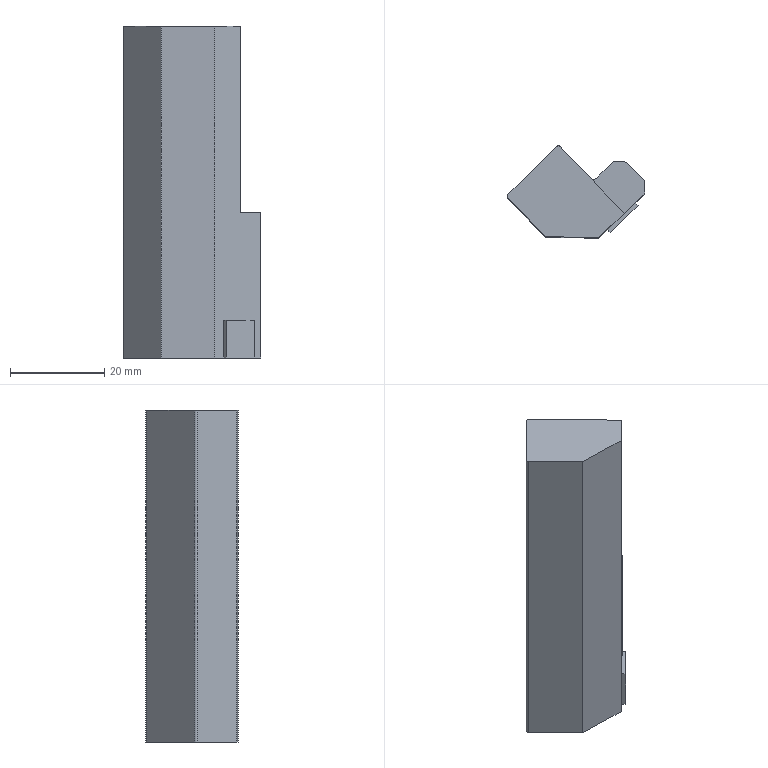Part | STEP file | gslz 2016.10.28-13_id1662_x_t | 1 solid | 19 faces | box 29.227 x 19.541 x 70.5 mm | volume 21986 mm3 | plane 16 | cylinder 3 | commonest cylinder face diameters 1 x2 2 x1
STEP:
#1=CARTESIAN_POINT('',(0.,0.,0.));
#2=DIRECTION('',(0.,0.,1.));
#3=DIRECTION('',(1.,0.,0.));
#4=AXIS2_PLACEMENT_3D('',#1,#2,#3);
#5=CARTESIAN_POINT('',(612.182,-228.399,-23.5));
#6=VERTEX_POINT('',#5);
#7=CARTESIAN_POINT('',(604.209,-220.085,-23.5));
#8=VERTEX_POINT('',#7);
#9=CARTESIAN_POINT('',(645.405,-263.044,-23.5));
#10=DIRECTION('',(-0.6921,0.7218,0.));
#11=VECTOR('',#10,1.);
#12=LINE('',#9,#11);
#13=CARTESIAN_POINT('',(-997.948,1450.63,-27.));
#14=DIRECTION('',(0.7218,0.6921,0.));
#15=DIRECTION('',(-0.6921,0.7218,0.));
#16=AXIS2_PLACEMENT_3D('',#13,#14,#15);
#17=PLANE('',#16);
#18=CARTESIAN_POINT('',(-2374.297,3.5));
#19=DIRECTION('',(1.,0.));
#20=VECTOR('',#19,1.);
#21=LINE('',#18,#20);
#22=(GEOMETRIC_REPRESENTATION_CONTEXT(2)PARAMETRIC_REPRESENTATION_CONTEXT()REPRESENTATION_CONTEXT('',''));
#23=DEFINITIONAL_REPRESENTATION('',(#21),#22);
#24=PCURVE('',#17,#23);
#25=CARTESIAN_POINT('',(467.733,-433.425,-23.5));
#26=DIRECTION('',(0.,0.,1.));
#27=DIRECTION('',(1.,0.,0.));
#28=AXIS2_PLACEMENT_3D('',#25,#26,#27);
#29=PLANE('',#28);
#30=CARTESIAN_POINT('',(177.672,170.382));
#31=DIRECTION('',(-0.6921,0.7218));
#32=VECTOR('',#31,1.);
#33=LINE('',#30,#32);
#34=(GEOMETRIC_REPRESENTATION_CONTEXT(2)PARAMETRIC_REPRESENTATION_CONTEXT()REPRESENTATION_CONTEXT('',''));
#35=DEFINITIONAL_REPRESENTATION('',(#33),#34);
#36=PCURVE('',#29,#35);
#37=SURFACE_CURVE('',#12,(#24,#36),.PCURVE_S1.);
#38=EDGE_CURVE('',#6,#8,#37,.T.);
#39=ORIENTED_EDGE('',*,*,#38,.T.);
#40=CARTESIAN_POINT('',(604.209,-220.085,-94.));
#41=VERTEX_POINT('',#40);
#42=CARTESIAN_POINT('',(604.209,-220.085,-94.));
#43=DIRECTION('',(0.,0.,-1.));
#44=VECTOR('',#43,1.);
#45=LINE('',#42,#44);
#46=CARTESIAN_POINT('',(-2314.777,-67.));
#47=DIRECTION('',(0.,-1.));
#48=VECTOR('',#47,1.);
#49=LINE('',#46,#48);
#50=(GEOMETRIC_REPRESENTATION_CONTEXT(2)PARAMETRIC_REPRESENTATION_CONTEXT()REPRESENTATION_CONTEXT('',''));
#51=DEFINITIONAL_REPRESENTATION('',(#49),#50);
#52=PCURVE('',#17,#51);
#53=CARTESIAN_POINT('',(604.57,-219.739,-116.74));
#54=DIRECTION('',(0.,0.,-1.));
#55=DIRECTION('',(-1.,0.,0.));
#56=AXIS2_PLACEMENT_3D('',#53,#54,#55);
#57=CYLINDRICAL_SURFACE('',#56,0.5);
#58=CARTESIAN_POINT('',(-0.7645,-22.74));
#59=DIRECTION('',(0.,1.));
#60=VECTOR('',#59,1.);
#61=LINE('',#58,#60);
#62=(GEOMETRIC_REPRESENTATION_CONTEXT(2)PARAMETRIC_REPRESENTATION_CONTEXT()REPRESENTATION_CONTEXT('',''));
#63=DEFINITIONAL_REPRESENTATION('',(#61),#62);
#64=PCURVE('',#57,#63);
#65=SURFACE_CURVE('',#45,(#52,#64),.PCURVE_S1.);
#66=EDGE_CURVE('',#8,#41,#65,.T.);
#67=ORIENTED_EDGE('',*,*,#66,.T.);
#68=CARTESIAN_POINT('',(612.182,-228.399,-94.));
#69=VERTEX_POINT('',#68);
#70=CARTESIAN_POINT('',(26.482,382.364,-94.));
#71=DIRECTION('',(-0.6921,0.7218,0.));
#72=VECTOR('',#71,1.);
#73=LINE('',#70,#72);
#74=CARTESIAN_POINT('',(-1480.084,-67.));
#75=DIRECTION('',(1.,0.));
#76=VECTOR('',#75,1.);
#77=LINE('',#74,#76);
#78=(GEOMETRIC_REPRESENTATION_CONTEXT(2)PARAMETRIC_REPRESENTATION_CONTEXT()REPRESENTATION_CONTEXT('',''));
#79=DEFINITIONAL_REPRESENTATION('',(#77),#78);
#80=PCURVE('',#17,#79);
#81=CARTESIAN_POINT('',(-151.191,211.982,-94.));
#82=DIRECTION('',(0.,0.,1.));
#83=DIRECTION('',(1.,0.,0.));
#84=AXIS2_PLACEMENT_3D('',#81,#82,#83);
#85=PLANE('',#84);
#86=CARTESIAN_POINT('',(177.672,170.382));
#87=DIRECTION('',(-0.6921,0.7218));
#88=VECTOR('',#87,1.);
#89=LINE('',#86,#88);
#90=(GEOMETRIC_REPRESENTATION_CONTEXT(2)PARAMETRIC_REPRESENTATION_CONTEXT()REPRESENTATION_CONTEXT('',''));
#91=DEFINITIONAL_REPRESENTATION('',(#89),#90);
#92=PCURVE('',#85,#91);
#93=SURFACE_CURVE('',#73,(#80,#92),.PCURVE_S1.);
#94=EDGE_CURVE('',#69,#41,#93,.T.);
#95=ORIENTED_EDGE('',*,*,#94,.F.);
#96=CARTESIAN_POINT('',(612.182,-228.399,-23.5));
#97=DIRECTION('',(0.,0.,1.));
#98=VECTOR('',#97,1.);
#99=LINE('',#96,#98);
#100=CARTESIAN_POINT('',(-2326.297,3.5));
#101=DIRECTION('',(0.,1.));
#102=VECTOR('',#101,1.);
#103=LINE('',#100,#102);
#104=(GEOMETRIC_REPRESENTATION_CONTEXT(2)PARAMETRIC_REPRESENTATION_CONTEXT()REPRESENTATION_CONTEXT('',''));
#105=DEFINITIONAL_REPRESENTATION('',(#103),#104);
#106=PCURVE('',#17,#105);
#107=CARTESIAN_POINT('',(612.182,-228.399,-27.));
#108=DIRECTION('',(-0.02094,-0.9998,0.));
#109=DIRECTION('',(0.,0.,-1.));
#110=AXIS2_PLACEMENT_3D('',#107,#108,#109);
#111=PLANE('',#110);
#112=CARTESIAN_POINT('',(-3.5,0.));
#113=DIRECTION('',(-1.,0.));
#114=VECTOR('',#113,1.);
#115=LINE('',#112,#114);
#116=(GEOMETRIC_REPRESENTATION_CONTEXT(2)PARAMETRIC_REPRESENTATION_CONTEXT()REPRESENTATION_CONTEXT('',''));
#117=DEFINITIONAL_REPRESENTATION('',(#115),#116);
#118=PCURVE('',#111,#117);
#119=SURFACE_CURVE('',#99,(#106,#118),.PCURVE_S1.);
#120=EDGE_CURVE('',#69,#6,#119,.T.);
#121=ORIENTED_EDGE('',*,*,#120,.T.);
#122=EDGE_LOOP('',(#39,#67,#95,#121));
#123=FACE_BOUND('',#122,.T.);
#124=ADVANCED_FACE('',(#123),#17,.F.);
#125=CARTESIAN_POINT('',(604.22,-219.381,-94.));
#126=VERTEX_POINT('',#125);
#127=CARTESIAN_POINT('',(604.57,-219.739,-94.));
#128=DIRECTION('',(0.,0.,-1.));
#129=DIRECTION('',(1.,0.,0.));
#130=AXIS2_PLACEMENT_3D('',#127,#128,#129);
#131=CIRCLE('',#130,0.5);
#132=CARTESIAN_POINT('',(-3.142,-22.74));
#133=DIRECTION('',(1.,0.));
#134=VECTOR('',#133,1.);
#135=LINE('',#132,#134);
#136=(GEOMETRIC_REPRESENTATION_CONTEXT(2)PARAMETRIC_REPRESENTATION_CONTEXT()REPRESENTATION_CONTEXT('',''));
#137=DEFINITIONAL_REPRESENTATION('',(#135),#136);
#138=PCURVE('',#57,#137);
#139=CARTESIAN_POINT('',(756.261,-431.721));
#140=CARTESIAN_POINT('',(756.261,-432.587));
#141=CARTESIAN_POINT('',(755.511,-432.154));
#142=CARTESIAN_POINT('',(754.761,-431.721));
#143=CARTESIAN_POINT('',(755.511,-431.288));
#144=CARTESIAN_POINT('',(756.261,-430.855));
#145=CARTESIAN_POINT('',(756.261,-431.721));
#146=(BOUNDED_CURVE()B_SPLINE_CURVE(2,(#139,#140,#141,#142,#143,#144,#145),.UNSPECIFIED.,.T.,.F.)B_SPLINE_CURVE_WITH_KNOTS((1,2,2,2,2,1),(-2.094,0.,2.094,4.189,6.283,8.378),.UNSPECIFIED.)CURVE()GEOMETRIC_REPRESENTATION_ITEM()RATIONAL_B_SPLINE_CURVE((1.,0.5,1.,0.5,1.,0.5,1.))REPRESENTATION_ITEM(''));
#147=(GEOMETRIC_REPRESENTATION_CONTEXT(2)PARAMETRIC_REPRESENTATION_CONTEXT()REPRESENTATION_CONTEXT('',''));
#148=DEFINITIONAL_REPRESENTATION('',(#146),#147);
#149=PCURVE('',#85,#148);
#150=SURFACE_CURVE('',#131,(#138,#149),.PCURVE_S1.);
#151=EDGE_CURVE('',#41,#126,#150,.T.);
#152=ORIENTED_EDGE('',*,*,#151,.F.);
#153=ORIENTED_EDGE('',*,*,#66,.F.);
#154=CARTESIAN_POINT('',(604.22,-219.381,-23.5));
#155=VERTEX_POINT('',#154);
#156=CARTESIAN_POINT('',(604.57,-219.739,-23.5));
#157=DIRECTION('',(0.,0.,1.));
#158=DIRECTION('',(1.,0.,0.));
#159=AXIS2_PLACEMENT_3D('',#156,#157,#158);
#160=CIRCLE('',#159,0.5);
#161=CARTESIAN_POINT('',(3.142,-93.24));
#162=DIRECTION('',(-1.,0.));
#163=VECTOR('',#162,1.);
#164=LINE('',#161,#163);
#165=(GEOMETRIC_REPRESENTATION_CONTEXT(2)PARAMETRIC_REPRESENTATION_CONTEXT()REPRESENTATION_CONTEXT('',''));
#166=DEFINITIONAL_REPRESENTATION('',(#164),#165);
#167=PCURVE('',#57,#166);
#168=CARTESIAN_POINT('',(136.837,213.687));
#169=DIRECTION('',(1.,0.));
#170=AXIS2_PLACEMENT_2D('',#168,#169);
#171=CIRCLE('',#170,0.5);
#172=(GEOMETRIC_REPRESENTATION_CONTEXT(2)PARAMETRIC_REPRESENTATION_CONTEXT()REPRESENTATION_CONTEXT('',''));
#173=DEFINITIONAL_REPRESENTATION('',(#171),#172);
#174=PCURVE('',#29,#173);
#175=SURFACE_CURVE('',#160,(#167,#174),.PCURVE_S1.);
#176=EDGE_CURVE('',#155,#8,#175,.T.);
#177=ORIENTED_EDGE('',*,*,#176,.F.);
#178=CARTESIAN_POINT('',(604.22,-219.381,-23.5));
#179=DIRECTION('',(0.,0.,1.));
#180=VECTOR('',#179,1.);
#181=LINE('',#178,#180);
#182=CARTESIAN_POINT('',(0.796,-93.24));
#183=DIRECTION('',(0.,-1.));
#184=VECTOR('',#183,1.);
#185=LINE('',#182,#184);
#186=(GEOMETRIC_REPRESENTATION_CONTEXT(2)PARAMETRIC_REPRESENTATION_CONTEXT()REPRESENTATION_CONTEXT('',''));
#187=DEFINITIONAL_REPRESENTATION('',(#185),#186);
#188=PCURVE('',#57,#187);
#189=CARTESIAN_POINT('',(622.374,-201.61,-116.74));
#190=DIRECTION('',(-0.6995,0.7146,0.));
#191=DIRECTION('',(-0.7146,-0.6995,0.));
#192=AXIS2_PLACEMENT_3D('',#189,#190,#191);
#193=PLANE('',#192);
#194=CARTESIAN_POINT('',(25.405,93.24));
#195=DIRECTION('',(0.,1.));
#196=VECTOR('',#195,1.);
#197=LINE('',#194,#196);
#198=(GEOMETRIC_REPRESENTATION_CONTEXT(2)PARAMETRIC_REPRESENTATION_CONTEXT()REPRESENTATION_CONTEXT('',''));
#199=DEFINITIONAL_REPRESENTATION('',(#197),#198);
#200=PCURVE('',#193,#199);
#201=SURFACE_CURVE('',#181,(#188,#200),.PCURVE_S1.);
#202=EDGE_CURVE('',#126,#155,#201,.T.);
#203=ORIENTED_EDGE('',*,*,#202,.F.);
#204=EDGE_LOOP('',(#152,#153,#177,#203));
#205=FACE_BOUND('',#204,.T.);
#206=ADVANCED_FACE('',(#205),#57,.T.);
#207=CARTESIAN_POINT('',(614.582,-209.237,-94.));
#208=VERTEX_POINT('',#207);
#209=CARTESIAN_POINT('',(434.109,-385.91,-94.));
#210=DIRECTION('',(-0.7146,-0.6995,0.));
#211=VECTOR('',#210,1.);
#212=LINE('',#209,#211);
#213=CARTESIAN_POINT('',(263.458,22.74));
#214=DIRECTION('',(1.,0.));
#215=VECTOR('',#214,1.);
#216=LINE('',#213,#215);
#217=(GEOMETRIC_REPRESENTATION_CONTEXT(2)PARAMETRIC_REPRESENTATION_CONTEXT()REPRESENTATION_CONTEXT('',''));
#218=DEFINITIONAL_REPRESENTATION('',(#216),#217);
#219=PCURVE('',#193,#218);
#220=CARTESIAN_POINT('',(585.3,-597.892));
#221=DIRECTION('',(-0.7146,-0.6995));
#222=VECTOR('',#221,1.);
#223=LINE('',#220,#222);
#224=(GEOMETRIC_REPRESENTATION_CONTEXT(2)PARAMETRIC_REPRESENTATION_CONTEXT()REPRESENTATION_CONTEXT('',''));
#225=DEFINITIONAL_REPRESENTATION('',(#223),#224);
#226=PCURVE('',#85,#225);
#227=SURFACE_CURVE('',#212,(#219,#226),.PCURVE_S1.);
#228=EDGE_CURVE('',#208,#126,#227,.T.);
#229=ORIENTED_EDGE('',*,*,#228,.T.);
#230=ORIENTED_EDGE('',*,*,#202,.T.);
#231=CARTESIAN_POINT('',(614.582,-209.237,-23.5));
#232=VERTEX_POINT('',#231);
#233=CARTESIAN_POINT('',(427.526,-392.354,-23.5));
#234=DIRECTION('',(-0.7146,-0.6995,0.));
#235=VECTOR('',#234,1.);
#236=LINE('',#233,#235);
#237=CARTESIAN_POINT('',(272.67,93.24));
#238=DIRECTION('',(1.,0.));
#239=VECTOR('',#238,1.);
#240=LINE('',#237,#239);
#241=(GEOMETRIC_REPRESENTATION_CONTEXT(2)PARAMETRIC_REPRESENTATION_CONTEXT()REPRESENTATION_CONTEXT('',''));
#242=DEFINITIONAL_REPRESENTATION('',(#240),#241);
#243=PCURVE('',#193,#242);
#244=CARTESIAN_POINT('',(-40.206,41.071));
#245=DIRECTION('',(-0.7146,-0.6995));
#246=VECTOR('',#245,1.);
#247=LINE('',#244,#246);
#248=(GEOMETRIC_REPRESENTATION_CONTEXT(2)PARAMETRIC_REPRESENTATION_CONTEXT()REPRESENTATION_CONTEXT('',''));
#249=DEFINITIONAL_REPRESENTATION('',(#247),#248);
#250=PCURVE('',#29,#249);
#251=SURFACE_CURVE('',#236,(#243,#250),.PCURVE_S1.);
#252=EDGE_CURVE('',#232,#155,#251,.T.);
#253=ORIENTED_EDGE('',*,*,#252,.F.);
#254=CARTESIAN_POINT('',(614.582,-209.237,-94.));
#255=DIRECTION('',(0.,0.,-1.));
#256=VECTOR('',#255,1.);
#257=LINE('',#254,#256);
#258=CARTESIAN_POINT('',(10.904,22.74));
#259=DIRECTION('',(0.,-1.));
#260=VECTOR('',#259,1.);
#261=LINE('',#258,#260);
#262=(GEOMETRIC_REPRESENTATION_CONTEXT(2)PARAMETRIC_REPRESENTATION_CONTEXT()REPRESENTATION_CONTEXT('',''));
#263=DEFINITIONAL_REPRESENTATION('',(#261),#262);
#264=PCURVE('',#193,#263);
#265=CARTESIAN_POINT('',(614.932,-209.595,-116.74));
#266=DIRECTION('',(0.,0.,1.));
#267=DIRECTION('',(1.,0.,0.));
#268=AXIS2_PLACEMENT_3D('',#265,#266,#267);
#269=CYLINDRICAL_SURFACE('',#268,0.5);
#270=CARTESIAN_POINT('',(2.346,22.74));
#271=DIRECTION('',(0.,-1.));
#272=VECTOR('',#271,1.);
#273=LINE('',#270,#272);
#274=(GEOMETRIC_REPRESENTATION_CONTEXT(2)PARAMETRIC_REPRESENTATION_CONTEXT()REPRESENTATION_CONTEXT('',''));
#275=DEFINITIONAL_REPRESENTATION('',(#273),#274);
#276=PCURVE('',#269,#275);
#277=SURFACE_CURVE('',#257,(#264,#276),.PCURVE_S1.);
#278=EDGE_CURVE('',#232,#208,#277,.T.);
#279=ORIENTED_EDGE('',*,*,#278,.T.);
#280=EDGE_LOOP('',(#229,#230,#253,#279));
#281=FACE_BOUND('',#280,.T.);
#282=ADVANCED_FACE('',(#281),#193,.T.);
#283=CARTESIAN_POINT('',(615.293,-209.249,-23.5));
#284=VERTEX_POINT('',#283);
#285=CARTESIAN_POINT('',(614.932,-209.595,-23.5));
#286=DIRECTION('',(0.,0.,1.));
#287=DIRECTION('',(1.,0.,0.));
#288=AXIS2_PLACEMENT_3D('',#285,#286,#287);
#289=CIRCLE('',#288,0.5);
#290=CARTESIAN_POINT('',(0.,93.24));
#291=DIRECTION('',(1.,0.));
#292=VECTOR('',#291,1.);
#293=LINE('',#290,#292);
#294=(GEOMETRIC_REPRESENTATION_CONTEXT(2)PARAMETRIC_REPRESENTATION_CONTEXT()REPRESENTATION_CONTEXT('',''));
#295=DEFINITIONAL_REPRESENTATION('',(#293),#294);
#296=PCURVE('',#269,#295);
#297=CARTESIAN_POINT('',(147.199,223.831));
#298=DIRECTION('',(1.,0.));
#299=AXIS2_PLACEMENT_2D('',#297,#298);
#300=CIRCLE('',#299,0.5);
#301=(GEOMETRIC_REPRESENTATION_CONTEXT(2)PARAMETRIC_REPRESENTATION_CONTEXT()REPRESENTATION_CONTEXT('',''));
#302=DEFINITIONAL_REPRESENTATION('',(#300),#301);
#303=PCURVE('',#29,#302);
#304=SURFACE_CURVE('',#289,(#296,#303),.PCURVE_S1.);
#305=EDGE_CURVE('',#284,#232,#304,.T.);
#306=ORIENTED_EDGE('',*,*,#305,.F.);
#307=CARTESIAN_POINT('',(615.293,-209.249,-94.));
#308=VERTEX_POINT('',#307);
#309=CARTESIAN_POINT('',(615.293,-209.249,-23.5));
#310=DIRECTION('',(0.,0.,1.));
#311=VECTOR('',#310,1.);
#312=LINE('',#309,#311);
#313=CARTESIAN_POINT('',(0.7645,93.24));
#314=DIRECTION('',(0.,1.));
#315=VECTOR('',#314,1.);
#316=LINE('',#313,#315);
#317=(GEOMETRIC_REPRESENTATION_CONTEXT(2)PARAMETRIC_REPRESENTATION_CONTEXT()REPRESENTATION_CONTEXT('',''));
#318=DEFINITIONAL_REPRESENTATION('',(#316),#317);
#319=PCURVE('',#269,#318);
#320=CARTESIAN_POINT('',(-986.761,1461.358,-27.));
#321=DIRECTION('',(-0.7218,-0.6921,0.));
#322=DIRECTION('',(0.6921,-0.7218,0.));
#323=AXIS2_PLACEMENT_3D('',#320,#321,#322);
#324=PLANE('',#323);
#325=CARTESIAN_POINT('',(2314.628,3.5));
#326=DIRECTION('',(0.,1.));
#327=VECTOR('',#326,1.);
#328=LINE('',#325,#327);
#329=(GEOMETRIC_REPRESENTATION_CONTEXT(2)PARAMETRIC_REPRESENTATION_CONTEXT()REPRESENTATION_CONTEXT('',''));
#330=DEFINITIONAL_REPRESENTATION('',(#328),#329);
#331=PCURVE('',#324,#330);
#332=SURFACE_CURVE('',#312,(#319,#331),.PCURVE_S1.);
#333=EDGE_CURVE('',#308,#284,#332,.T.);
#334=ORIENTED_EDGE('',*,*,#333,.F.);
#335=CARTESIAN_POINT('',(614.932,-209.595,-94.));
#336=DIRECTION('',(0.,0.,-1.));
#337=DIRECTION('',(1.,0.,0.));
#338=AXIS2_PLACEMENT_3D('',#335,#336,#337);
#339=CIRCLE('',#338,0.5);
#340=CARTESIAN_POINT('',(6.283,22.74));
#341=DIRECTION('',(-1.,0.));
#342=VECTOR('',#341,1.);
#343=LINE('',#340,#342);
#344=(GEOMETRIC_REPRESENTATION_CONTEXT(2)PARAMETRIC_REPRESENTATION_CONTEXT()REPRESENTATION_CONTEXT('',''));
#345=DEFINITIONAL_REPRESENTATION('',(#343),#344);
#346=PCURVE('',#269,#345);
#347=CARTESIAN_POINT('',(766.623,-421.577));
#348=CARTESIAN_POINT('',(766.623,-422.443));
#349=CARTESIAN_POINT('',(765.873,-422.01));
#350=CARTESIAN_POINT('',(765.123,-421.577));
#351=CARTESIAN_POINT('',(765.873,-421.144));
#352=CARTESIAN_POINT('',(766.623,-420.711));
#353=CARTESIAN_POINT('',(766.623,-421.577));
#354=(BOUNDED_CURVE()B_SPLINE_CURVE(2,(#347,#348,#349,#350,#351,#352,#353),.UNSPECIFIED.,.T.,.F.)B_SPLINE_CURVE_WITH_KNOTS((1,2,2,2,2,1),(-2.094,0.,2.094,4.189,6.283,8.378),.UNSPECIFIED.)CURVE()GEOMETRIC_REPRESENTATION_ITEM()RATIONAL_B_SPLINE_CURVE((1.,0.5,1.,0.5,1.,0.5,1.))REPRESENTATION_ITEM(''));
#355=(GEOMETRIC_REPRESENTATION_CONTEXT(2)PARAMETRIC_REPRESENTATION_CONTEXT()REPRESENTATION_CONTEXT('',''));
#356=DEFINITIONAL_REPRESENTATION('',(#354),#355);
#357=PCURVE('',#85,#356);
#358=SURFACE_CURVE('',#339,(#346,#357),.PCURVE_S1.);
#359=EDGE_CURVE('',#208,#308,#358,.T.);
#360=ORIENTED_EDGE('',*,*,#359,.F.);
#361=ORIENTED_EDGE('',*,*,#278,.F.);
#362=EDGE_LOOP('',(#306,#334,#360,#361));
#363=FACE_BOUND('',#362,.T.);
#364=ADVANCED_FACE('',(#363),#269,.T.);
#365=CARTESIAN_POINT('',(623.494,-228.636,-94.));
#366=VERTEX_POINT('',#365);
#367=CARTESIAN_POINT('',(612.182,-228.399,-94.));
#368=DIRECTION('',(-0.9998,0.02094,0.));
#369=VECTOR('',#368,1.);
#370=LINE('',#367,#369);
#371=CARTESIAN_POINT('',(67.,0.));
#372=DIRECTION('',(0.,-1.));
#373=VECTOR('',#372,1.);
#374=LINE('',#371,#373);
#375=(GEOMETRIC_REPRESENTATION_CONTEXT(2)PARAMETRIC_REPRESENTATION_CONTEXT()REPRESENTATION_CONTEXT('',''));
#376=DEFINITIONAL_REPRESENTATION('',(#374),#375);
#377=PCURVE('',#111,#376);
#378=CARTESIAN_POINT('',(763.373,-440.381));
#379=DIRECTION('',(-0.9998,0.02094));
#380=VECTOR('',#379,1.);
#381=LINE('',#378,#380);
#382=(GEOMETRIC_REPRESENTATION_CONTEXT(2)PARAMETRIC_REPRESENTATION_CONTEXT()REPRESENTATION_CONTEXT('',''));
#383=DEFINITIONAL_REPRESENTATION('',(#381),#382);
#384=PCURVE('',#85,#383);
#385=SURFACE_CURVE('',#370,(#377,#384),.PCURVE_S1.);
#386=EDGE_CURVE('',#366,#69,#385,.T.);
#387=ORIENTED_EDGE('',*,*,#386,.F.);
#388=CARTESIAN_POINT('',(623.494,-228.636,-23.5));
#389=VERTEX_POINT('',#388);
#390=CARTESIAN_POINT('',(623.494,-228.636,-94.));
#391=DIRECTION('',(0.,0.,-1.));
#392=VECTOR('',#391,1.);
#393=LINE('',#390,#392);
#394=CARTESIAN_POINT('',(67.,11.314));
#395=DIRECTION('',(1.,0.));
#396=VECTOR('',#395,1.);
#397=LINE('',#394,#396);
#398=(GEOMETRIC_REPRESENTATION_CONTEXT(2)PARAMETRIC_REPRESENTATION_CONTEXT()REPRESENTATION_CONTEXT('',''));
#399=DEFINITIONAL_REPRESENTATION('',(#397),#398);
#400=PCURVE('',#111,#399);
#401=CARTESIAN_POINT('',(95.668,-734.803,-27.));
#402=DIRECTION('',(0.6921,-0.7218,0.));
#403=DIRECTION('',(0.7218,0.6921,0.));
#404=AXIS2_PLACEMENT_3D('',#401,#402,#403);
#405=PLANE('',#404);
#406=CARTESIAN_POINT('',(731.303,-67.));
#407=DIRECTION('',(0.,-1.));
#408=VECTOR('',#407,1.);
#409=LINE('',#406,#408);
#410=(GEOMETRIC_REPRESENTATION_CONTEXT(2)PARAMETRIC_REPRESENTATION_CONTEXT()REPRESENTATION_CONTEXT('',''));
#411=DEFINITIONAL_REPRESENTATION('',(#409),#410);
#412=PCURVE('',#405,#411);
#413=SURFACE_CURVE('',#393,(#400,#412),.PCURVE_S1.);
#414=EDGE_CURVE('',#389,#366,#413,.T.);
#415=ORIENTED_EDGE('',*,*,#414,.F.);
#416=CARTESIAN_POINT('',(472.089,-225.465,-23.5));
#417=DIRECTION('',(0.9998,-0.02094,0.));
#418=VECTOR('',#417,1.);
#419=LINE('',#416,#418);
#420=CARTESIAN_POINT('',(-3.5,-140.124));
#421=DIRECTION('',(0.,1.));
#422=VECTOR('',#421,1.);
#423=LINE('',#420,#422);
#424=(GEOMETRIC_REPRESENTATION_CONTEXT(2)PARAMETRIC_REPRESENTATION_CONTEXT()REPRESENTATION_CONTEXT('',''));
#425=DEFINITIONAL_REPRESENTATION('',(#423),#424);
#426=PCURVE('',#111,#425);
#427=CARTESIAN_POINT('',(4.356,207.961));
#428=DIRECTION('',(0.9998,-0.02094));
#429=VECTOR('',#428,1.);
#430=LINE('',#427,#429);
#431=(GEOMETRIC_REPRESENTATION_CONTEXT(2)PARAMETRIC_REPRESENTATION_CONTEXT()REPRESENTATION_CONTEXT('',''));
#432=DEFINITIONAL_REPRESENTATION('',(#430),#431);
#433=PCURVE('',#29,#432);
#434=SURFACE_CURVE('',#419,(#426,#433),.PCURVE_S1.);
#435=EDGE_CURVE('',#6,#389,#434,.T.);
#436=ORIENTED_EDGE('',*,*,#435,.F.);
#437=ORIENTED_EDGE('',*,*,#120,.F.);
#438=EDGE_LOOP('',(#387,#415,#436,#437));
#439=FACE_BOUND('',#438,.T.);
#440=ADVANCED_FACE('',(#439),#111,.T.);
#441=CARTESIAN_POINT('',(625.406,-226.802,-94.));
#442=VERTEX_POINT('',#441);
#443=CARTESIAN_POINT('',(625.406,-226.802,-86.));
#444=VERTEX_POINT('',#443);
#445=CARTESIAN_POINT('',(625.406,-226.802,-27.));
#446=DIRECTION('',(0.,0.,1.));
#447=VECTOR('',#446,1.);
#448=LINE('',#445,#447);
#449=CARTESIAN_POINT('',(625.96,-227.379,-27.));
#450=DIRECTION('',(-0.7218,-0.6921,0.));
#451=DIRECTION('',(0.6921,-0.7218,0.));
#452=AXIS2_PLACEMENT_3D('',#449,#450,#451);
#453=PLANE('',#452);
#454=CARTESIAN_POINT('',(-0.8,0.));
#455=DIRECTION('',(0.,1.));
#456=VECTOR('',#455,1.);
#457=LINE('',#454,#456);
#458=(GEOMETRIC_REPRESENTATION_CONTEXT(2)PARAMETRIC_REPRESENTATION_CONTEXT()REPRESENTATION_CONTEXT('',''));
#459=DEFINITIONAL_REPRESENTATION('',(#457),#458);
#460=PCURVE('',#453,#459);
#461=CARTESIAN_POINT('',(733.953,0.));
#462=DIRECTION('',(0.,1.));
#463=VECTOR('',#462,1.);
#464=LINE('',#461,#463);
#465=(GEOMETRIC_REPRESENTATION_CONTEXT(2)PARAMETRIC_REPRESENTATION_CONTEXT()REPRESENTATION_CONTEXT('',''));
#466=DEFINITIONAL_REPRESENTATION('',(#464),#465);
#467=PCURVE('',#405,#466);
#468=SURFACE_CURVE('',#448,(#460,#467),.PCURVE_S1.);
#469=EDGE_CURVE('',#442,#444,#468,.T.);
#470=ORIENTED_EDGE('',*,*,#469,.F.);
#471=CARTESIAN_POINT('',(625.96,-227.379,-94.));
#472=VERTEX_POINT('',#471);
#473=CARTESIAN_POINT('',(625.96,-227.379,-94.));
#474=DIRECTION('',(-0.6921,0.7218,0.));
#475=VECTOR('',#474,1.);
#476=LINE('',#473,#475);
#477=CARTESIAN_POINT('',(0.,-67.));
#478=DIRECTION('',(-1.,0.));
#479=VECTOR('',#478,1.);
#480=LINE('',#477,#479);
#481=(GEOMETRIC_REPRESENTATION_CONTEXT(2)PARAMETRIC_REPRESENTATION_CONTEXT()REPRESENTATION_CONTEXT('',''));
#482=DEFINITIONAL_REPRESENTATION('',(#480),#481);
#483=PCURVE('',#453,#482);
#484=CARTESIAN_POINT('',(777.151,-439.362));
#485=DIRECTION('',(-0.6921,0.7218));
#486=VECTOR('',#485,1.);
#487=LINE('',#484,#486);
#488=(GEOMETRIC_REPRESENTATION_CONTEXT(2)PARAMETRIC_REPRESENTATION_CONTEXT()REPRESENTATION_CONTEXT('',''));
#489=DEFINITIONAL_REPRESENTATION('',(#487),#488);
#490=PCURVE('',#85,#489);
#491=SURFACE_CURVE('',#476,(#483,#490),.PCURVE_S1.);
#492=EDGE_CURVE('',#472,#442,#491,.T.);
#493=ORIENTED_EDGE('',*,*,#492,.F.);
#494=CARTESIAN_POINT('',(625.96,-227.379,-86.));
#495=VERTEX_POINT('',#494);
#496=CARTESIAN_POINT('',(625.96,-227.379,-27.));
#497=DIRECTION('',(0.,0.,1.));
#498=VECTOR('',#497,1.);
#499=LINE('',#496,#498);
#500=CARTESIAN_POINT('',(0.,0.));
#501=DIRECTION('',(0.,1.));
#502=VECTOR('',#501,1.);
#503=LINE('',#500,#502);
#504=(GEOMETRIC_REPRESENTATION_CONTEXT(2)PARAMETRIC_REPRESENTATION_CONTEXT()REPRESENTATION_CONTEXT('',''));
#505=DEFINITIONAL_REPRESENTATION('',(#503),#504);
#506=PCURVE('',#453,#505);
#507=CARTESIAN_POINT('',(96.222,-735.38,-27.));
#508=DIRECTION('',(0.6921,-0.7218,0.));
#509=DIRECTION('',(0.7218,0.6921,0.));
#510=AXIS2_PLACEMENT_3D('',#507,#508,#509);
#511=PLANE('',#510);
#512=CARTESIAN_POINT('',(733.953,0.));
#513=DIRECTION('',(0.,1.));
#514=VECTOR('',#513,1.);
#515=LINE('',#512,#514);
#516=(GEOMETRIC_REPRESENTATION_CONTEXT(2)PARAMETRIC_REPRESENTATION_CONTEXT()REPRESENTATION_CONTEXT('',''));
#517=DEFINITIONAL_REPRESENTATION('',(#515),#516);
#518=PCURVE('',#511,#517);
#519=SURFACE_CURVE('',#499,(#506,#518),.PCURVE_S1.);
#520=EDGE_CURVE('',#472,#495,#519,.T.);
#521=ORIENTED_EDGE('',*,*,#520,.T.);
#522=CARTESIAN_POINT('',(625.96,-227.379,-86.));
#523=DIRECTION('',(-0.6921,0.7218,0.));
#524=VECTOR('',#523,1.);
#525=LINE('',#522,#524);
#526=CARTESIAN_POINT('',(0.,-59.));
#527=DIRECTION('',(-1.,0.));
#528=VECTOR('',#527,1.);
#529=LINE('',#526,#528);
#530=(GEOMETRIC_REPRESENTATION_CONTEXT(2)PARAMETRIC_REPRESENTATION_CONTEXT()REPRESENTATION_CONTEXT('',''));
#531=DEFINITIONAL_REPRESENTATION('',(#529),#530);
#532=PCURVE('',#453,#531);
#533=CARTESIAN_POINT('',(-151.191,211.982,-86.));
#534=DIRECTION('',(0.,0.,1.));
#535=DIRECTION('',(1.,0.,0.));
#536=AXIS2_PLACEMENT_3D('',#533,#534,#535);
#537=PLANE('',#536);
#538=CARTESIAN_POINT('',(777.151,-439.362));
#539=DIRECTION('',(-0.6921,0.7218));
#540=VECTOR('',#539,1.);
#541=LINE('',#538,#540);
#542=(GEOMETRIC_REPRESENTATION_CONTEXT(2)PARAMETRIC_REPRESENTATION_CONTEXT()REPRESENTATION_CONTEXT('',''));
#543=DEFINITIONAL_REPRESENTATION('',(#541),#542);
#544=PCURVE('',#537,#543);
#545=SURFACE_CURVE('',#525,(#532,#544),.PCURVE_S1.);
#546=EDGE_CURVE('',#495,#444,#545,.T.);
#547=ORIENTED_EDGE('',*,*,#546,.T.);
#548=EDGE_LOOP('',(#470,#493,#521,#547));
#549=FACE_BOUND('',#548,.T.);
#550=ADVANCED_FACE('',(#549),#453,.T.);
#551=CARTESIAN_POINT('',(628.907,-223.445,-63.));
#552=VERTEX_POINT('',#551);
#553=CARTESIAN_POINT('',(628.907,-223.445,-23.5));
#554=VERTEX_POINT('',#553);
#555=CARTESIAN_POINT('',(628.907,-223.445,-27.));
#556=DIRECTION('',(0.,0.,1.));
#557=VECTOR('',#556,1.);
#558=LINE('',#555,#557);
#559=CARTESIAN_POINT('',(2334.297,0.));
#560=DIRECTION('',(0.,1.));
#561=VECTOR('',#560,1.);
#562=LINE('',#559,#561);
#563=(GEOMETRIC_REPRESENTATION_CONTEXT(2)PARAMETRIC_REPRESENTATION_CONTEXT()REPRESENTATION_CONTEXT('',''));
#564=DEFINITIONAL_REPRESENTATION('',(#562),#563);
#565=PCURVE('',#324,#564);
#566=CARTESIAN_POINT('',(738.803,0.));
#567=DIRECTION('',(0.,1.));
#568=VECTOR('',#567,1.);
#569=LINE('',#566,#568);
#570=(GEOMETRIC_REPRESENTATION_CONTEXT(2)PARAMETRIC_REPRESENTATION_CONTEXT()REPRESENTATION_CONTEXT('',''));
#571=DEFINITIONAL_REPRESENTATION('',(#569),#570);
#572=PCURVE('',#405,#571);
#573=SURFACE_CURVE('',#558,(#565,#572),.PCURVE_S1.);
#574=EDGE_CURVE('',#552,#554,#573,.T.);
#575=ORIENTED_EDGE('',*,*,#574,.F.);
#576=CARTESIAN_POINT('',(621.639,-215.866,-63.));
#577=VERTEX_POINT('',#576);
#578=CARTESIAN_POINT('',(644.432,-239.634,-63.));
#579=DIRECTION('',(-0.6921,0.7218,0.));
#580=VECTOR('',#579,1.);
#581=LINE('',#578,#580);
#582=CARTESIAN_POINT('',(2356.728,-36.));
#583=DIRECTION('',(-1.,0.));
#584=VECTOR('',#583,1.);
#585=LINE('',#582,#584);
#586=(GEOMETRIC_REPRESENTATION_CONTEXT(2)PARAMETRIC_REPRESENTATION_CONTEXT()REPRESENTATION_CONTEXT('',''));
#587=DEFINITIONAL_REPRESENTATION('',(#585),#586);
#588=PCURVE('',#324,#587);
#589=CARTESIAN_POINT('',(462.091,-414.493,-63.));
#590=DIRECTION('',(0.,0.,-1.));
#591=DIRECTION('',(-1.,0.,0.));
#592=AXIS2_PLACEMENT_3D('',#589,#590,#591);
#593=PLANE('',#592);
#594=CARTESIAN_POINT('',(-182.341,174.859));
#595=DIRECTION('',(0.6921,0.7218));
#596=VECTOR('',#595,1.);
#597=LINE('',#594,#596);
#598=(GEOMETRIC_REPRESENTATION_CONTEXT(2)PARAMETRIC_REPRESENTATION_CONTEXT()REPRESENTATION_CONTEXT('',''));
#599=DEFINITIONAL_REPRESENTATION('',(#597),#598);
#600=PCURVE('',#593,#599);
#601=SURFACE_CURVE('',#581,(#588,#600),.PCURVE_S1.);
#602=EDGE_CURVE('',#552,#577,#601,.T.);
#603=ORIENTED_EDGE('',*,*,#602,.T.);
#604=CARTESIAN_POINT('',(621.639,-215.866,-94.));
#605=VERTEX_POINT('',#604);
#606=CARTESIAN_POINT('',(621.639,-215.866,-27.));
#607=DIRECTION('',(0.,0.,1.));
#608=VECTOR('',#607,1.);
#609=LINE('',#606,#608);
#610=CARTESIAN_POINT('',(2323.797,0.));
#611=DIRECTION('',(0.,1.));
#612=VECTOR('',#611,1.);
#613=LINE('',#610,#612);
#614=(GEOMETRIC_REPRESENTATION_CONTEXT(2)PARAMETRIC_REPRESENTATION_CONTEXT()REPRESENTATION_CONTEXT('',''));
#615=DEFINITIONAL_REPRESENTATION('',(#613),#614);
#616=PCURVE('',#324,#615);
#617=CARTESIAN_POINT('',(622.361,-215.174,-27.));
#618=DIRECTION('',(0.,0.,1.));
#619=DIRECTION('',(1.,0.,0.));
#620=AXIS2_PLACEMENT_3D('',#617,#618,#619);
#621=CYLINDRICAL_SURFACE('',#620,1.);
#622=CARTESIAN_POINT('',(3.906,0.));
#623=DIRECTION('',(0.,1.));
#624=VECTOR('',#623,1.);
#625=LINE('',#622,#624);
#626=(GEOMETRIC_REPRESENTATION_CONTEXT(2)PARAMETRIC_REPRESENTATION_CONTEXT()REPRESENTATION_CONTEXT('',''));
#627=DEFINITIONAL_REPRESENTATION('',(#625),#626);
#628=PCURVE('',#621,#627);
#629=SURFACE_CURVE('',#609,(#616,#628),.PCURVE_S1.);
#630=EDGE_CURVE('',#605,#577,#629,.T.);
#631=ORIENTED_EDGE('',*,*,#630,.F.);
#632=CARTESIAN_POINT('',(37.669,393.092,-94.));
#633=DIRECTION('',(0.6921,-0.7218,0.));
#634=VECTOR('',#633,1.);
#635=LINE('',#632,#634);
#636=CARTESIAN_POINT('',(1480.084,-67.));
#637=DIRECTION('',(1.,0.));
#638=VECTOR('',#637,1.);
#639=LINE('',#636,#638);
#640=(GEOMETRIC_REPRESENTATION_CONTEXT(2)PARAMETRIC_REPRESENTATION_CONTEXT()REPRESENTATION_CONTEXT('',''));
#641=DEFINITIONAL_REPRESENTATION('',(#639),#640);
#642=PCURVE('',#324,#641);
#643=CARTESIAN_POINT('',(188.86,181.11));
#644=DIRECTION('',(0.6921,-0.7218));
#645=VECTOR('',#644,1.);
#646=LINE('',#643,#645);
#647=(GEOMETRIC_REPRESENTATION_CONTEXT(2)PARAMETRIC_REPRESENTATION_CONTEXT()REPRESENTATION_CONTEXT('',''));
#648=DEFINITIONAL_REPRESENTATION('',(#646),#647);
#649=PCURVE('',#85,#648);
#650=SURFACE_CURVE('',#635,(#642,#649),.PCURVE_S1.);
#651=EDGE_CURVE('',#308,#605,#650,.T.);
#652=ORIENTED_EDGE('',*,*,#651,.F.);
#653=ORIENTED_EDGE('',*,*,#333,.T.);
#654=CARTESIAN_POINT('',(656.592,-252.315,-23.5));
#655=DIRECTION('',(0.6921,-0.7218,0.));
#656=VECTOR('',#655,1.);
#657=LINE('',#654,#656);
#658=CARTESIAN_POINT('',(2374.297,3.5));
#659=DIRECTION('',(1.,0.));
#660=VECTOR('',#659,1.);
#661=LINE('',#658,#660);
#662=(GEOMETRIC_REPRESENTATION_CONTEXT(2)PARAMETRIC_REPRESENTATION_CONTEXT()REPRESENTATION_CONTEXT('',''));
#663=DEFINITIONAL_REPRESENTATION('',(#661),#662);
#664=PCURVE('',#324,#663);
#665=CARTESIAN_POINT('',(188.86,181.11));
#666=DIRECTION('',(0.6921,-0.7218));
#667=VECTOR('',#666,1.);
#668=LINE('',#665,#667);
#669=(GEOMETRIC_REPRESENTATION_CONTEXT(2)PARAMETRIC_REPRESENTATION_CONTEXT()REPRESENTATION_CONTEXT('',''));
#670=DEFINITIONAL_REPRESENTATION('',(#668),#669);
#671=PCURVE('',#29,#670);
#672=SURFACE_CURVE('',#657,(#664,#671),.PCURVE_S1.);
#673=EDGE_CURVE('',#284,#554,#672,.T.);
#674=ORIENTED_EDGE('',*,*,#673,.T.);
#675=EDGE_LOOP('',(#575,#603,#631,#652,#653,#674));
#676=FACE_BOUND('',#675,.T.);
#677=ADVANCED_FACE('',(#676),#324,.F.);
#678=CARTESIAN_POINT('',(631.878,-221.704,-94.));
#679=VERTEX_POINT('',#678);
#680=CARTESIAN_POINT('',(440.601,-405.132,-94.));
#681=DIRECTION('',(0.7218,0.6921,0.));
#682=VECTOR('',#681,1.);
#683=LINE('',#680,#682);
#684=CARTESIAN_POINT('',(477.138,-67.));
#685=DIRECTION('',(1.,0.));
#686=VECTOR('',#685,1.);
#687=LINE('',#684,#686);
#688=(GEOMETRIC_REPRESENTATION_CONTEXT(2)PARAMETRIC_REPRESENTATION_CONTEXT()REPRESENTATION_CONTEXT('',''));
#689=DEFINITIONAL_REPRESENTATION('',(#687),#688);
#690=PCURVE('',#511,#689);
#691=CARTESIAN_POINT('',(591.792,-617.115));
#692=DIRECTION('',(0.7218,0.6921));
#693=VECTOR('',#692,1.);
#694=LINE('',#691,#693);
#695=(GEOMETRIC_REPRESENTATION_CONTEXT(2)PARAMETRIC_REPRESENTATION_CONTEXT()REPRESENTATION_CONTEXT('',''));
#696=DEFINITIONAL_REPRESENTATION('',(#694),#695);
#697=PCURVE('',#85,#696);
#698=SURFACE_CURVE('',#683,(#690,#697),.PCURVE_S1.);
#699=EDGE_CURVE('',#472,#679,#698,.T.);
#700=ORIENTED_EDGE('',*,*,#699,.T.);
#701=CARTESIAN_POINT('',(631.878,-221.704,-86.));
#702=VERTEX_POINT('',#701);
#703=CARTESIAN_POINT('',(631.878,-221.704,-27.));
#704=DIRECTION('',(0.,0.,1.));
#705=VECTOR('',#704,1.);
#706=LINE('',#703,#705);
#707=CARTESIAN_POINT('',(742.153,0.));
#708=DIRECTION('',(0.,1.));
#709=VECTOR('',#708,1.);
#710=LINE('',#707,#709);
#711=(GEOMETRIC_REPRESENTATION_CONTEXT(2)PARAMETRIC_REPRESENTATION_CONTEXT()REPRESENTATION_CONTEXT('',''));
#712=DEFINITIONAL_REPRESENTATION('',(#710),#711);
#713=PCURVE('',#511,#712);
#714=CARTESIAN_POINT('',(631.878,-221.704,-27.));
#715=DIRECTION('',(-0.7218,-0.6921,0.));
#716=DIRECTION('',(0.6921,-0.7218,0.));
#717=AXIS2_PLACEMENT_3D('',#714,#715,#716);
#718=PLANE('',#717);
#719=CARTESIAN_POINT('',(0.,0.));
#720=DIRECTION('',(0.,1.));
#721=VECTOR('',#720,1.);
#722=LINE('',#719,#721);
#723=(GEOMETRIC_REPRESENTATION_CONTEXT(2)PARAMETRIC_REPRESENTATION_CONTEXT()REPRESENTATION_CONTEXT('',''));
#724=DEFINITIONAL_REPRESENTATION('',(#722),#723);
#725=PCURVE('',#718,#724);
#726=SURFACE_CURVE('',#706,(#713,#725),.PCURVE_S1.);
#727=EDGE_CURVE('',#679,#702,#726,.T.);
#728=ORIENTED_EDGE('',*,*,#727,.T.);
#729=CARTESIAN_POINT('',(440.601,-405.132,-86.));
#730=DIRECTION('',(0.7218,0.6921,0.));
#731=VECTOR('',#730,1.);
#732=LINE('',#729,#731);
#733=CARTESIAN_POINT('',(477.138,-59.));
#734=DIRECTION('',(1.,0.));
#735=VECTOR('',#734,1.);
#736=LINE('',#733,#735);
#737=(GEOMETRIC_REPRESENTATION_CONTEXT(2)PARAMETRIC_REPRESENTATION_CONTEXT()REPRESENTATION_CONTEXT('',''));
#738=DEFINITIONAL_REPRESENTATION('',(#736),#737);
#739=PCURVE('',#511,#738);
#740=CARTESIAN_POINT('',(591.792,-617.115));
#741=DIRECTION('',(0.7218,0.6921));
#742=VECTOR('',#741,1.);
#743=LINE('',#740,#742);
#744=(GEOMETRIC_REPRESENTATION_CONTEXT(2)PARAMETRIC_REPRESENTATION_CONTEXT()REPRESENTATION_CONTEXT('',''));
#745=DEFINITIONAL_REPRESENTATION('',(#743),#744);
#746=PCURVE('',#537,#745);
#747=SURFACE_CURVE('',#732,(#739,#746),.PCURVE_S1.);
#748=EDGE_CURVE('',#495,#702,#747,.T.);
#749=ORIENTED_EDGE('',*,*,#748,.F.);
#750=ORIENTED_EDGE('',*,*,#520,.F.);
#751=EDGE_LOOP('',(#700,#728,#749,#750));
#752=FACE_BOUND('',#751,.T.);
#753=ADVANCED_FACE('',(#752),#511,.T.);
#754=ORIENTED_EDGE('',*,*,#748,.T.);
#755=CARTESIAN_POINT('',(631.325,-221.126,-86.));
#756=VERTEX_POINT('',#755);
#757=CARTESIAN_POINT('',(631.878,-221.704,-86.));
#758=DIRECTION('',(-0.6921,0.7218,0.));
#759=VECTOR('',#758,1.);
#760=LINE('',#757,#759);
#761=CARTESIAN_POINT('',(783.069,-433.686));
#762=DIRECTION('',(-0.6921,0.7218));
#763=VECTOR('',#762,1.);
#764=LINE('',#761,#763);
#765=(GEOMETRIC_REPRESENTATION_CONTEXT(2)PARAMETRIC_REPRESENTATION_CONTEXT()REPRESENTATION_CONTEXT('',''));
#766=DEFINITIONAL_REPRESENTATION('',(#764),#765);
#767=PCURVE('',#537,#766);
#768=CARTESIAN_POINT('',(0.,-59.));
#769=DIRECTION('',(-1.,0.));
#770=VECTOR('',#769,1.);
#771=LINE('',#768,#770);
#772=(GEOMETRIC_REPRESENTATION_CONTEXT(2)PARAMETRIC_REPRESENTATION_CONTEXT()REPRESENTATION_CONTEXT('',''));
#773=DEFINITIONAL_REPRESENTATION('',(#771),#772);
#774=PCURVE('',#718,#773);
#775=SURFACE_CURVE('',#760,(#767,#774),.PCURVE_S1.);
#776=EDGE_CURVE('',#702,#756,#775,.T.);
#777=ORIENTED_EDGE('',*,*,#776,.T.);
#778=CARTESIAN_POINT('',(440.047,-404.555,-86.));
#779=DIRECTION('',(0.7218,0.6921,0.));
#780=VECTOR('',#779,1.);
#781=LINE('',#778,#780);
#782=CARTESIAN_POINT('',(591.238,-616.537));
#783=DIRECTION('',(0.7218,0.6921));
#784=VECTOR('',#783,1.);
#785=LINE('',#782,#784);
#786=(GEOMETRIC_REPRESENTATION_CONTEXT(2)PARAMETRIC_REPRESENTATION_CONTEXT()REPRESENTATION_CONTEXT('',''));
#787=DEFINITIONAL_REPRESENTATION('',(#785),#786);
#788=PCURVE('',#537,#787);
#789=CARTESIAN_POINT('',(477.138,-59.));
#790=DIRECTION('',(1.,0.));
#791=VECTOR('',#790,1.);
#792=LINE('',#789,#791);
#793=(GEOMETRIC_REPRESENTATION_CONTEXT(2)PARAMETRIC_REPRESENTATION_CONTEXT()REPRESENTATION_CONTEXT('',''));
#794=DEFINITIONAL_REPRESENTATION('',(#792),#793);
#795=PCURVE('',#405,#794);
#796=SURFACE_CURVE('',#781,(#788,#795),.PCURVE_S1.);
#797=EDGE_CURVE('',#444,#756,#796,.T.);
#798=ORIENTED_EDGE('',*,*,#797,.F.);
#799=ORIENTED_EDGE('',*,*,#546,.F.);
#800=EDGE_LOOP('',(#754,#777,#798,#799));
#801=FACE_BOUND('',#800,.T.);
#802=ADVANCED_FACE('',(#801),#537,.T.);
#803=ORIENTED_EDGE('',*,*,#797,.T.);
#804=CARTESIAN_POINT('',(631.325,-221.126,-94.));
#805=VERTEX_POINT('',#804);
#806=CARTESIAN_POINT('',(631.325,-221.126,-27.));
#807=DIRECTION('',(0.,0.,1.));
#808=VECTOR('',#807,1.);
#809=LINE('',#806,#808);
#810=CARTESIAN_POINT('',(742.153,0.));
#811=DIRECTION('',(0.,1.));
#812=VECTOR('',#811,1.);
#813=LINE('',#810,#812);
#814=(GEOMETRIC_REPRESENTATION_CONTEXT(2)PARAMETRIC_REPRESENTATION_CONTEXT()REPRESENTATION_CONTEXT('',''));
#815=DEFINITIONAL_REPRESENTATION('',(#813),#814);
#816=PCURVE('',#405,#815);
#817=CARTESIAN_POINT('',(-0.8,0.));
#818=DIRECTION('',(0.,1.));
#819=VECTOR('',#818,1.);
#820=LINE('',#817,#819);
#821=(GEOMETRIC_REPRESENTATION_CONTEXT(2)PARAMETRIC_REPRESENTATION_CONTEXT()REPRESENTATION_CONTEXT('',''));
#822=DEFINITIONAL_REPRESENTATION('',(#820),#821);
#823=PCURVE('',#718,#822);
#824=SURFACE_CURVE('',#809,(#816,#823),.PCURVE_S1.);
#825=EDGE_CURVE('',#805,#756,#824,.T.);
#826=ORIENTED_EDGE('',*,*,#825,.F.);
#827=CARTESIAN_POINT('',(633.237,-219.292,-94.));
#828=VERTEX_POINT('',#827);
#829=CARTESIAN_POINT('',(440.047,-404.555,-94.));
#830=DIRECTION('',(0.7218,0.6921,0.));
#831=VECTOR('',#830,1.);
#832=LINE('',#829,#831);
#833=CARTESIAN_POINT('',(477.138,-67.));
#834=DIRECTION('',(1.,0.));
#835=VECTOR('',#834,1.);
#836=LINE('',#833,#835);
#837=(GEOMETRIC_REPRESENTATION_CONTEXT(2)PARAMETRIC_REPRESENTATION_CONTEXT()REPRESENTATION_CONTEXT('',''));
#838=DEFINITIONAL_REPRESENTATION('',(#836),#837);
#839=PCURVE('',#405,#838);
#840=CARTESIAN_POINT('',(591.238,-616.537));
#841=DIRECTION('',(0.7218,0.6921));
#842=VECTOR('',#841,1.);
#843=LINE('',#840,#842);
#844=(GEOMETRIC_REPRESENTATION_CONTEXT(2)PARAMETRIC_REPRESENTATION_CONTEXT()REPRESENTATION_CONTEXT('',''));
#845=DEFINITIONAL_REPRESENTATION('',(#843),#844);
#846=PCURVE('',#85,#845);
#847=SURFACE_CURVE('',#832,(#839,#846),.PCURVE_S1.);
#848=EDGE_CURVE('',#805,#828,#847,.T.);
#849=ORIENTED_EDGE('',*,*,#848,.T.);
#850=CARTESIAN_POINT('',(633.237,-219.292,-63.));
#851=VERTEX_POINT('',#850);
#852=CARTESIAN_POINT('',(633.237,-219.292,-27.));
#853=DIRECTION('',(0.,0.,1.));
#854=VECTOR('',#853,1.);
#855=LINE('',#852,#854);
#856=CARTESIAN_POINT('',(744.803,0.));
#857=DIRECTION('',(0.,1.));
#858=VECTOR('',#857,1.);
#859=LINE('',#856,#858);
#860=(GEOMETRIC_REPRESENTATION_CONTEXT(2)PARAMETRIC_REPRESENTATION_CONTEXT()REPRESENTATION_CONTEXT('',''));
#861=DEFINITIONAL_REPRESENTATION('',(#859),#860);
#862=PCURVE('',#405,#861);
#863=CARTESIAN_POINT('',(633.237,-219.292,-27.));
#864=DIRECTION('',(-0.9998,0.02094,0.));
#865=DIRECTION('',(0.,0.,1.));
#866=AXIS2_PLACEMENT_3D('',#863,#864,#865);
#867=PLANE('',#866);
#868=CARTESIAN_POINT('',(0.,0.));
#869=DIRECTION('',(1.,0.));
#870=VECTOR('',#869,1.);
#871=LINE('',#868,#870);
#872=(GEOMETRIC_REPRESENTATION_CONTEXT(2)PARAMETRIC_REPRESENTATION_CONTEXT()REPRESENTATION_CONTEXT('',''));
#873=DEFINITIONAL_REPRESENTATION('',(#871),#872);
#874=PCURVE('',#867,#873);
#875=SURFACE_CURVE('',#855,(#862,#874),.PCURVE_S1.);
#876=EDGE_CURVE('',#828,#851,#875,.T.);
#877=ORIENTED_EDGE('',*,*,#876,.T.);
#878=CARTESIAN_POINT('',(446.566,-398.304,-63.));
#879=DIRECTION('',(0.7218,0.6921,0.));
#880=VECTOR('',#879,1.);
#881=LINE('',#878,#880);
#882=CARTESIAN_POINT('',(486.17,-36.));
#883=DIRECTION('',(1.,0.));
#884=VECTOR('',#883,1.);
#885=LINE('',#882,#884);
#886=(GEOMETRIC_REPRESENTATION_CONTEXT(2)PARAMETRIC_REPRESENTATION_CONTEXT()REPRESENTATION_CONTEXT('',''));
#887=DEFINITIONAL_REPRESENTATION('',(#885),#886);
#888=PCURVE('',#405,#887);
#889=CARTESIAN_POINT('',(15.525,16.19));
#890=DIRECTION('',(-0.7218,0.6921));
#891=VECTOR('',#890,1.);
#892=LINE('',#889,#891);
#893=(GEOMETRIC_REPRESENTATION_CONTEXT(2)PARAMETRIC_REPRESENTATION_CONTEXT()REPRESENTATION_CONTEXT('',''));
#894=DEFINITIONAL_REPRESENTATION('',(#892),#893);
#895=PCURVE('',#593,#894);
#896=SURFACE_CURVE('',#881,(#888,#895),.PCURVE_S1.);
#897=EDGE_CURVE('',#552,#851,#896,.T.);
#898=ORIENTED_EDGE('',*,*,#897,.F.);
#899=ORIENTED_EDGE('',*,*,#574,.T.);
#900=CARTESIAN_POINT('',(440.047,-404.555,-23.5));
#901=DIRECTION('',(0.7218,0.6921,0.));
#902=VECTOR('',#901,1.);
#903=LINE('',#900,#902);
#904=CARTESIAN_POINT('',(477.138,3.5));
#905=DIRECTION('',(1.,0.));
#906=VECTOR('',#905,1.);
#907=LINE('',#904,#906);
#908=(GEOMETRIC_REPRESENTATION_CONTEXT(2)PARAMETRIC_REPRESENTATION_CONTEXT()REPRESENTATION_CONTEXT('',''));
#909=DEFINITIONAL_REPRESENTATION('',(#907),#908);
#910=PCURVE('',#405,#909);
#911=CARTESIAN_POINT('',(-27.686,28.87));
#912=DIRECTION('',(0.7218,0.6921));
#913=VECTOR('',#912,1.);
#914=LINE('',#911,#913);
#915=(GEOMETRIC_REPRESENTATION_CONTEXT(2)PARAMETRIC_REPRESENTATION_CONTEXT()REPRESENTATION_CONTEXT('',''));
#916=DEFINITIONAL_REPRESENTATION('',(#914),#915);
#917=PCURVE('',#29,#916);
#918=SURFACE_CURVE('',#903,(#910,#917),.PCURVE_S1.);
#919=EDGE_CURVE('',#389,#554,#918,.T.);
#920=ORIENTED_EDGE('',*,*,#919,.F.);
#921=ORIENTED_EDGE('',*,*,#414,.T.);
#922=CARTESIAN_POINT('',(440.047,-404.555,-94.));
#923=DIRECTION('',(0.7218,0.6921,0.));
#924=VECTOR('',#923,1.);
#925=LINE('',#922,#924);
#926=CARTESIAN_POINT('',(477.138,-67.));
#927=DIRECTION('',(1.,0.));
#928=VECTOR('',#927,1.);
#929=LINE('',#926,#928);
#930=(GEOMETRIC_REPRESENTATION_CONTEXT(2)PARAMETRIC_REPRESENTATION_CONTEXT()REPRESENTATION_CONTEXT('',''));
#931=DEFINITIONAL_REPRESENTATION('',(#929),#930);
#932=PCURVE('',#405,#931);
#933=CARTESIAN_POINT('',(591.238,-616.537));
#934=DIRECTION('',(0.7218,0.6921));
#935=VECTOR('',#934,1.);
#936=LINE('',#933,#935);
#937=(GEOMETRIC_REPRESENTATION_CONTEXT(2)PARAMETRIC_REPRESENTATION_CONTEXT()REPRESENTATION_CONTEXT('',''));
#938=DEFINITIONAL_REPRESENTATION('',(#936),#937);
#939=PCURVE('',#85,#938);
#940=SURFACE_CURVE('',#925,(#932,#939),.PCURVE_S1.);
#941=EDGE_CURVE('',#366,#442,#940,.T.);
#942=ORIENTED_EDGE('',*,*,#941,.T.);
#943=ORIENTED_EDGE('',*,*,#469,.T.);
#944=EDGE_LOOP('',(#803,#826,#849,#877,#898,#899,#920,#921,#942,#943));
#945=FACE_BOUND('',#944,.T.);
#946=ADVANCED_FACE('',(#945),#405,.T.);
#947=ORIENTED_EDGE('',*,*,#919,.T.);
#948=ORIENTED_EDGE('',*,*,#673,.F.);
#949=ORIENTED_EDGE('',*,*,#305,.T.);
#950=ORIENTED_EDGE('',*,*,#252,.T.);
#951=ORIENTED_EDGE('',*,*,#176,.T.);
#952=ORIENTED_EDGE('',*,*,#38,.F.);
#953=ORIENTED_EDGE('',*,*,#435,.T.);
#954=EDGE_LOOP('',(#947,#948,#949,#950,#951,#952,#953));
#955=FACE_BOUND('',#954,.T.);
#956=ADVANCED_FACE('',(#955),#29,.T.);
#957=ORIENTED_EDGE('',*,*,#651,.T.);
#958=CARTESIAN_POINT('',(623.053,-215.896,-94.));
#959=VERTEX_POINT('',#958);
#960=CARTESIAN_POINT('',(622.361,-215.174,-94.));
#961=DIRECTION('',(0.,0.,-1.));
#962=DIRECTION('',(1.,0.,0.));
#963=AXIS2_PLACEMENT_3D('',#960,#961,#962);
#964=CIRCLE('',#963,1.);
#965=CARTESIAN_POINT('',(774.552,-427.157));
#966=CARTESIAN_POINT('',(774.552,-428.889));
#967=CARTESIAN_POINT('',(773.052,-428.023));
#968=CARTESIAN_POINT('',(771.552,-427.157));
#969=CARTESIAN_POINT('',(773.052,-426.291));
#970=CARTESIAN_POINT('',(774.552,-425.425));
#971=CARTESIAN_POINT('',(774.552,-427.157));
#972=(BOUNDED_CURVE()B_SPLINE_CURVE(2,(#965,#966,#967,#968,#969,#970,#971),.UNSPECIFIED.,.T.,.F.)B_SPLINE_CURVE_WITH_KNOTS((1,2,2,2,2,1),(-2.094,0.,2.094,4.189,6.283,8.378),.UNSPECIFIED.)CURVE()GEOMETRIC_REPRESENTATION_ITEM()RATIONAL_B_SPLINE_CURVE((1.,0.5,1.,0.5,1.,0.5,1.))REPRESENTATION_ITEM(''));
#973=(GEOMETRIC_REPRESENTATION_CONTEXT(2)PARAMETRIC_REPRESENTATION_CONTEXT()REPRESENTATION_CONTEXT('',''));
#974=DEFINITIONAL_REPRESENTATION('',(#972),#973);
#975=PCURVE('',#85,#974);
#976=CARTESIAN_POINT('',(6.283,-67.));
#977=DIRECTION('',(-1.,0.));
#978=VECTOR('',#977,1.);
#979=LINE('',#976,#978);
#980=(GEOMETRIC_REPRESENTATION_CONTEXT(2)PARAMETRIC_REPRESENTATION_CONTEXT()REPRESENTATION_CONTEXT('',''));
#981=DEFINITIONAL_REPRESENTATION('',(#979),#980);
#982=PCURVE('',#621,#981);
#983=SURFACE_CURVE('',#964,(#975,#982),.PCURVE_S1.);
#984=EDGE_CURVE('',#959,#605,#983,.T.);
#985=ORIENTED_EDGE('',*,*,#984,.F.);
#986=CARTESIAN_POINT('',(626.662,-212.435,-94.));
#987=VERTEX_POINT('',#986);
#988=CARTESIAN_POINT('',(433.472,-397.698,-94.));
#989=DIRECTION('',(-0.7218,-0.6921,0.));
#990=VECTOR('',#989,1.);
#991=LINE('',#988,#990);
#992=CARTESIAN_POINT('',(584.663,-609.68));
#993=DIRECTION('',(-0.7218,-0.6921));
#994=VECTOR('',#993,1.);
#995=LINE('',#992,#994);
#996=(GEOMETRIC_REPRESENTATION_CONTEXT(2)PARAMETRIC_REPRESENTATION_CONTEXT()REPRESENTATION_CONTEXT('',''));
#997=DEFINITIONAL_REPRESENTATION('',(#995),#996);
#998=PCURVE('',#85,#997);
#999=CARTESIAN_POINT('',(89.092,-727.946,-27.));
#1000=DIRECTION('',(-0.6921,0.7218,0.));
#1001=DIRECTION('',(-0.7218,-0.6921,0.));
#1002=AXIS2_PLACEMENT_3D('',#999,#1000,#1001);
#1003=PLANE('',#1002);
#1004=CARTESIAN_POINT('',(-477.138,-67.));
#1005=DIRECTION('',(1.,0.));
#1006=VECTOR('',#1005,1.);
#1007=LINE('',#1004,#1006);
#1008=(GEOMETRIC_REPRESENTATION_CONTEXT(2)PARAMETRIC_REPRESENTATION_CONTEXT()REPRESENTATION_CONTEXT('',''));
#1009=DEFINITIONAL_REPRESENTATION('',(#1007),#1008);
#1010=PCURVE('',#1003,#1009);
#1011=SURFACE_CURVE('',#991,(#998,#1010),.PCURVE_S1.);
#1012=EDGE_CURVE('',#987,#959,#1011,.T.);
#1013=ORIENTED_EDGE('',*,*,#1012,.F.);
#1014=CARTESIAN_POINT('',(629.49,-212.495,-94.));
#1015=VERTEX_POINT('',#1014);
#1016=CARTESIAN_POINT('',(629.49,-212.495,-94.));
#1017=DIRECTION('',(0.9998,-0.02094,0.));
#1018=VECTOR('',#1017,1.);
#1019=LINE('',#1016,#1018);
#1020=CARTESIAN_POINT('',(780.681,-424.477));
#1021=DIRECTION('',(0.9998,-0.02094));
#1022=VECTOR('',#1021,1.);
#1023=LINE('',#1020,#1022);
#1024=(GEOMETRIC_REPRESENTATION_CONTEXT(2)PARAMETRIC_REPRESENTATION_CONTEXT()REPRESENTATION_CONTEXT('',''));
#1025=DEFINITIONAL_REPRESENTATION('',(#1023),#1024);
#1026=PCURVE('',#85,#1025);
#1027=CARTESIAN_POINT('',(629.49,-212.495,-27.));
#1028=DIRECTION('',(-0.02094,-0.9998,0.));
#1029=DIRECTION('',(0.,0.,1.));
#1030=AXIS2_PLACEMENT_3D('',#1027,#1028,#1029);
#1031=PLANE('',#1030);
#1032=CARTESIAN_POINT('',(-67.,0.));
#1033=DIRECTION('',(0.,-1.));
#1034=VECTOR('',#1033,1.);
#1035=LINE('',#1032,#1034);
#1036=(GEOMETRIC_REPRESENTATION_CONTEXT(2)PARAMETRIC_REPRESENTATION_CONTEXT()REPRESENTATION_CONTEXT('',''));
#1037=DEFINITIONAL_REPRESENTATION('',(#1035),#1036);
#1038=PCURVE('',#1031,#1037);
#1039=SURFACE_CURVE('',#1019,(#1026,#1038),.PCURVE_S1.);
#1040=EDGE_CURVE('',#987,#1015,#1039,.T.);
#1041=ORIENTED_EDGE('',*,*,#1040,.T.);
#1042=CARTESIAN_POINT('',(633.297,-216.464,-94.));
#1043=VERTEX_POINT('',#1042);
#1044=CARTESIAN_POINT('',(43.443,398.629,-94.));
#1045=DIRECTION('',(-0.6921,0.7218,0.));
#1046=VECTOR('',#1045,1.);
#1047=LINE('',#1044,#1046);
#1048=CARTESIAN_POINT('',(194.634,186.647));
#1049=DIRECTION('',(-0.6921,0.7218));
#1050=VECTOR('',#1049,1.);
#1051=LINE('',#1048,#1050);
#1052=(GEOMETRIC_REPRESENTATION_CONTEXT(2)PARAMETRIC_REPRESENTATION_CONTEXT()REPRESENTATION_CONTEXT('',''));
#1053=DEFINITIONAL_REPRESENTATION('',(#1051),#1052);
#1054=PCURVE('',#85,#1053);
#1055=CARTESIAN_POINT('',(-980.987,1466.895,-27.));
#1056=DIRECTION('',(0.7218,0.6921,0.));
#1057=DIRECTION('',(-0.6921,0.7218,0.));
#1058=AXIS2_PLACEMENT_3D('',#1055,#1056,#1057);
#1059=PLANE('',#1058);
#1060=CARTESIAN_POINT('',(-1480.084,-67.));
#1061=DIRECTION('',(1.,0.));
#1062=VECTOR('',#1061,1.);
#1063=LINE('',#1060,#1062);
#1064=(GEOMETRIC_REPRESENTATION_CONTEXT(2)PARAMETRIC_REPRESENTATION_CONTEXT()REPRESENTATION_CONTEXT('',''));
#1065=DEFINITIONAL_REPRESENTATION('',(#1063),#1064);
#1066=PCURVE('',#1059,#1065);
#1067=SURFACE_CURVE('',#1047,(#1054,#1066),.PCURVE_S1.);
#1068=EDGE_CURVE('',#1043,#1015,#1067,.T.);
#1069=ORIENTED_EDGE('',*,*,#1068,.F.);
#1070=CARTESIAN_POINT('',(633.237,-219.292,-94.));
#1071=DIRECTION('',(-0.02094,-0.9998,0.));
#1072=VECTOR('',#1071,1.);
#1073=LINE('',#1070,#1072);
#1074=CARTESIAN_POINT('',(784.428,-431.274));
#1075=DIRECTION('',(-0.02094,-0.9998));
#1076=VECTOR('',#1075,1.);
#1077=LINE('',#1074,#1076);
#1078=(GEOMETRIC_REPRESENTATION_CONTEXT(2)PARAMETRIC_REPRESENTATION_CONTEXT()REPRESENTATION_CONTEXT('',''));
#1079=DEFINITIONAL_REPRESENTATION('',(#1077),#1078);
#1080=PCURVE('',#85,#1079);
#1081=CARTESIAN_POINT('',(-67.,0.));
#1082=DIRECTION('',(0.,-1.));
#1083=VECTOR('',#1082,1.);
#1084=LINE('',#1081,#1083);
#1085=(GEOMETRIC_REPRESENTATION_CONTEXT(2)PARAMETRIC_REPRESENTATION_CONTEXT()REPRESENTATION_CONTEXT('',''));
#1086=DEFINITIONAL_REPRESENTATION('',(#1084),#1085);
#1087=PCURVE('',#867,#1086);
#1088=SURFACE_CURVE('',#1073,(#1080,#1087),.PCURVE_S1.);
#1089=EDGE_CURVE('',#1043,#828,#1088,.T.);
#1090=ORIENTED_EDGE('',*,*,#1089,.T.);
#1091=ORIENTED_EDGE('',*,*,#848,.F.);
#1092=CARTESIAN_POINT('',(631.878,-221.704,-94.));
#1093=DIRECTION('',(-0.6921,0.7218,0.));
#1094=VECTOR('',#1093,1.);
#1095=LINE('',#1092,#1094);
#1096=CARTESIAN_POINT('',(783.069,-433.686));
#1097=DIRECTION('',(-0.6921,0.7218));
#1098=VECTOR('',#1097,1.);
#1099=LINE('',#1096,#1098);
#1100=(GEOMETRIC_REPRESENTATION_CONTEXT(2)PARAMETRIC_REPRESENTATION_CONTEXT()REPRESENTATION_CONTEXT('',''));
#1101=DEFINITIONAL_REPRESENTATION('',(#1099),#1100);
#1102=PCURVE('',#85,#1101);
#1103=CARTESIAN_POINT('',(0.,-67.));
#1104=DIRECTION('',(-1.,0.));
#1105=VECTOR('',#1104,1.);
#1106=LINE('',#1103,#1105);
#1107=(GEOMETRIC_REPRESENTATION_CONTEXT(2)PARAMETRIC_REPRESENTATION_CONTEXT()REPRESENTATION_CONTEXT('',''));
#1108=DEFINITIONAL_REPRESENTATION('',(#1106),#1107);
#1109=PCURVE('',#718,#1108);
#1110=SURFACE_CURVE('',#1095,(#1102,#1109),.PCURVE_S1.);
#1111=EDGE_CURVE('',#679,#805,#1110,.T.);
#1112=ORIENTED_EDGE('',*,*,#1111,.F.);
#1113=ORIENTED_EDGE('',*,*,#699,.F.);
#1114=ORIENTED_EDGE('',*,*,#492,.T.);
#1115=ORIENTED_EDGE('',*,*,#941,.F.);
#1116=ORIENTED_EDGE('',*,*,#386,.T.);
#1117=ORIENTED_EDGE('',*,*,#94,.T.);
#1118=ORIENTED_EDGE('',*,*,#151,.T.);
#1119=ORIENTED_EDGE('',*,*,#228,.F.);
#1120=ORIENTED_EDGE('',*,*,#359,.T.);
#1121=EDGE_LOOP('',(#957,#985,#1013,#1041,#1069,#1090,#1091,#1112,#1113,#1114,#1115,#1116,#1117,#1118,#1119,#1120));
#1122=FACE_BOUND('',#1121,.T.);
#1123=ADVANCED_FACE('',(#1122),#85,.F.);
#1124=ORIENTED_EDGE('',*,*,#602,.F.);
#1125=ORIENTED_EDGE('',*,*,#897,.T.);
#1126=CARTESIAN_POINT('',(633.297,-216.464,-63.));
#1127=VERTEX_POINT('',#1126);
#1128=CARTESIAN_POINT('',(629.075,-417.991,-63.));
#1129=DIRECTION('',(0.02094,0.9998,0.));
#1130=VECTOR('',#1129,1.);
#1131=LINE('',#1128,#1130);
#1132=CARTESIAN_POINT('',(-166.984,-3.498));
#1133=DIRECTION('',(-0.02094,0.9998));
#1134=VECTOR('',#1133,1.);
#1135=LINE('',#1132,#1134);
#1136=(GEOMETRIC_REPRESENTATION_CONTEXT(2)PARAMETRIC_REPRESENTATION_CONTEXT()REPRESENTATION_CONTEXT('',''));
#1137=DEFINITIONAL_REPRESENTATION('',(#1135),#1136);
#1138=PCURVE('',#593,#1137);
#1139=CARTESIAN_POINT('',(-36.,-198.743));
#1140=DIRECTION('',(0.,1.));
#1141=VECTOR('',#1140,1.);
#1142=LINE('',#1139,#1141);
#1143=(GEOMETRIC_REPRESENTATION_CONTEXT(2)PARAMETRIC_REPRESENTATION_CONTEXT()REPRESENTATION_CONTEXT('',''));
#1144=DEFINITIONAL_REPRESENTATION('',(#1142),#1143);
#1145=PCURVE('',#867,#1144);
#1146=SURFACE_CURVE('',#1131,(#1138,#1145),.PCURVE_S1.);
#1147=EDGE_CURVE('',#851,#1127,#1146,.T.);
#1148=ORIENTED_EDGE('',*,*,#1147,.T.);
#1149=CARTESIAN_POINT('',(629.49,-212.495,-63.));
#1150=VERTEX_POINT('',#1149);
#1151=CARTESIAN_POINT('',(650.206,-234.097,-63.));
#1152=DIRECTION('',(-0.6921,0.7218,0.));
#1153=VECTOR('',#1152,1.);
#1154=LINE('',#1151,#1153);
#1155=CARTESIAN_POINT('',(-188.115,180.396));
#1156=DIRECTION('',(0.6921,0.7218));
#1157=VECTOR('',#1156,1.);
#1158=LINE('',#1155,#1157);
#1159=(GEOMETRIC_REPRESENTATION_CONTEXT(2)PARAMETRIC_REPRESENTATION_CONTEXT()REPRESENTATION_CONTEXT('',''));
#1160=DEFINITIONAL_REPRESENTATION('',(#1158),#1159);
#1161=PCURVE('',#593,#1160);
#1162=CARTESIAN_POINT('',(-2356.728,-36.));
#1163=DIRECTION('',(1.,0.));
#1164=VECTOR('',#1163,1.);
#1165=LINE('',#1162,#1164);
#1166=(GEOMETRIC_REPRESENTATION_CONTEXT(2)PARAMETRIC_REPRESENTATION_CONTEXT()REPRESENTATION_CONTEXT('',''));
#1167=DEFINITIONAL_REPRESENTATION('',(#1165),#1166);
#1168=PCURVE('',#1059,#1167);
#1169=SURFACE_CURVE('',#1154,(#1161,#1168),.PCURVE_S1.);
#1170=EDGE_CURVE('',#1127,#1150,#1169,.T.);
#1171=ORIENTED_EDGE('',*,*,#1170,.T.);
#1172=CARTESIAN_POINT('',(626.662,-212.435,-63.));
#1173=VERTEX_POINT('',#1172);
#1174=CARTESIAN_POINT('',(466.394,-209.078,-63.));
#1175=DIRECTION('',(-0.9998,0.02094,0.));
#1176=VECTOR('',#1175,1.);
#1177=LINE('',#1174,#1176);
#1178=CARTESIAN_POINT('',(-4.303,205.415));
#1179=DIRECTION('',(0.9998,0.02094));
#1180=VECTOR('',#1179,1.);
#1181=LINE('',#1178,#1180);
#1182=(GEOMETRIC_REPRESENTATION_CONTEXT(2)PARAMETRIC_REPRESENTATION_CONTEXT()REPRESENTATION_CONTEXT('',''));
#1183=DEFINITIONAL_REPRESENTATION('',(#1181),#1182);
#1184=PCURVE('',#593,#1183);
#1185=CARTESIAN_POINT('',(-36.,163.132));
#1186=DIRECTION('',(0.,1.));
#1187=VECTOR('',#1186,1.);
#1188=LINE('',#1185,#1187);
#1189=(GEOMETRIC_REPRESENTATION_CONTEXT(2)PARAMETRIC_REPRESENTATION_CONTEXT()REPRESENTATION_CONTEXT('',''));
#1190=DEFINITIONAL_REPRESENTATION('',(#1188),#1189);
#1191=PCURVE('',#1031,#1190);
#1192=SURFACE_CURVE('',#1177,(#1184,#1191),.PCURVE_S1.);
#1193=EDGE_CURVE('',#1150,#1173,#1192,.T.);
#1194=ORIENTED_EDGE('',*,*,#1193,.T.);
#1195=CARTESIAN_POINT('',(623.053,-215.896,-63.));
#1196=VERTEX_POINT('',#1195);
#1197=CARTESIAN_POINT('',(439.99,-391.447,-63.));
#1198=DIRECTION('',(-0.7218,-0.6921,0.));
#1199=VECTOR('',#1198,1.);
#1200=LINE('',#1197,#1199);
#1201=CARTESIAN_POINT('',(22.101,23.046));
#1202=DIRECTION('',(0.7218,-0.6921));
#1203=VECTOR('',#1202,1.);
#1204=LINE('',#1201,#1203);
#1205=(GEOMETRIC_REPRESENTATION_CONTEXT(2)PARAMETRIC_REPRESENTATION_CONTEXT()REPRESENTATION_CONTEXT('',''));
#1206=DEFINITIONAL_REPRESENTATION('',(#1204),#1205);
#1207=PCURVE('',#593,#1206);
#1208=CARTESIAN_POINT('',(-486.17,-36.));
#1209=DIRECTION('',(1.,0.));
#1210=VECTOR('',#1209,1.);
#1211=LINE('',#1208,#1210);
#1212=(GEOMETRIC_REPRESENTATION_CONTEXT(2)PARAMETRIC_REPRESENTATION_CONTEXT()REPRESENTATION_CONTEXT('',''));
#1213=DEFINITIONAL_REPRESENTATION('',(#1211),#1212);
#1214=PCURVE('',#1003,#1213);
#1215=SURFACE_CURVE('',#1200,(#1207,#1214),.PCURVE_S1.);
#1216=EDGE_CURVE('',#1173,#1196,#1215,.T.);
#1217=ORIENTED_EDGE('',*,*,#1216,.T.);
#1218=CARTESIAN_POINT('',(622.361,-215.174,-63.));
#1219=DIRECTION('',(0.,0.,-1.));
#1220=DIRECTION('',(-1.,0.,0.));
#1221=AXIS2_PLACEMENT_3D('',#1218,#1219,#1220);
#1222=CIRCLE('',#1221,1.);
#1223=CARTESIAN_POINT('',(-160.27,199.319));
#1224=DIRECTION('',(1.,0.));
#1225=AXIS2_PLACEMENT_2D('',#1223,#1224);
#1226=CIRCLE('',#1225,1.);
#1227=(GEOMETRIC_REPRESENTATION_CONTEXT(2)PARAMETRIC_REPRESENTATION_CONTEXT()REPRESENTATION_CONTEXT('',''));
#1228=DEFINITIONAL_REPRESENTATION('',(#1226),#1227);
#1229=PCURVE('',#593,#1228);
#1230=CARTESIAN_POINT('',(9.425,-36.));
#1231=DIRECTION('',(-1.,0.));
#1232=VECTOR('',#1231,1.);
#1233=LINE('',#1230,#1232);
#1234=(GEOMETRIC_REPRESENTATION_CONTEXT(2)PARAMETRIC_REPRESENTATION_CONTEXT()REPRESENTATION_CONTEXT('',''));
#1235=DEFINITIONAL_REPRESENTATION('',(#1233),#1234);
#1236=PCURVE('',#621,#1235);
#1237=SURFACE_CURVE('',#1222,(#1229,#1236),.PCURVE_S1.);
#1238=EDGE_CURVE('',#1196,#577,#1237,.T.);
#1239=ORIENTED_EDGE('',*,*,#1238,.T.);
#1240=EDGE_LOOP('',(#1124,#1125,#1148,#1171,#1194,#1217,#1239));
#1241=FACE_BOUND('',#1240,.T.);
#1242=ADVANCED_FACE('',(#1241),#593,.F.);
#1243=ORIENTED_EDGE('',*,*,#1068,.T.);
#1244=CARTESIAN_POINT('',(629.49,-212.495,-27.));
#1245=DIRECTION('',(0.,0.,1.));
#1246=VECTOR('',#1245,1.);
#1247=LINE('',#1244,#1246);
#1248=CARTESIAN_POINT('',(-2326.797,0.));
#1249=DIRECTION('',(0.,1.));
#1250=VECTOR('',#1249,1.);
#1251=LINE('',#1248,#1250);
#1252=(GEOMETRIC_REPRESENTATION_CONTEXT(2)PARAMETRIC_REPRESENTATION_CONTEXT()REPRESENTATION_CONTEXT('',''));
#1253=DEFINITIONAL_REPRESENTATION('',(#1251),#1252);
#1254=PCURVE('',#1059,#1253);
#1255=CARTESIAN_POINT('',(0.,0.));
#1256=DIRECTION('',(1.,0.));
#1257=VECTOR('',#1256,1.);
#1258=LINE('',#1255,#1257);
#1259=(GEOMETRIC_REPRESENTATION_CONTEXT(2)PARAMETRIC_REPRESENTATION_CONTEXT()REPRESENTATION_CONTEXT('',''));
#1260=DEFINITIONAL_REPRESENTATION('',(#1258),#1259);
#1261=PCURVE('',#1031,#1260);
#1262=SURFACE_CURVE('',#1247,(#1254,#1261),.PCURVE_S1.);
#1263=EDGE_CURVE('',#1015,#1150,#1262,.T.);
#1264=ORIENTED_EDGE('',*,*,#1263,.T.);
#1265=ORIENTED_EDGE('',*,*,#1170,.F.);
#1266=CARTESIAN_POINT('',(633.297,-216.464,-27.));
#1267=DIRECTION('',(0.,0.,-1.));
#1268=VECTOR('',#1267,1.);
#1269=LINE('',#1266,#1268);
#1270=CARTESIAN_POINT('',(-2332.297,0.));
#1271=DIRECTION('',(0.,-1.));
#1272=VECTOR('',#1271,1.);
#1273=LINE('',#1270,#1272);
#1274=(GEOMETRIC_REPRESENTATION_CONTEXT(2)PARAMETRIC_REPRESENTATION_CONTEXT()REPRESENTATION_CONTEXT('',''));
#1275=DEFINITIONAL_REPRESENTATION('',(#1273),#1274);
#1276=PCURVE('',#1059,#1275);
#1277=CARTESIAN_POINT('',(0.,2.828));
#1278=DIRECTION('',(-1.,0.));
#1279=VECTOR('',#1278,1.);
#1280=LINE('',#1277,#1279);
#1281=(GEOMETRIC_REPRESENTATION_CONTEXT(2)PARAMETRIC_REPRESENTATION_CONTEXT()REPRESENTATION_CONTEXT('',''));
#1282=DEFINITIONAL_REPRESENTATION('',(#1280),#1281);
#1283=PCURVE('',#867,#1282);
#1284=SURFACE_CURVE('',#1269,(#1276,#1283),.PCURVE_S1.);
#1285=EDGE_CURVE('',#1127,#1043,#1284,.T.);
#1286=ORIENTED_EDGE('',*,*,#1285,.T.);
#1287=EDGE_LOOP('',(#1243,#1264,#1265,#1286));
#1288=FACE_BOUND('',#1287,.T.);
#1289=ADVANCED_FACE('',(#1288),#1059,.T.);
#1290=ORIENTED_EDGE('',*,*,#1216,.F.);
#1291=CARTESIAN_POINT('',(626.662,-212.435,-27.));
#1292=DIRECTION('',(0.,0.,-1.));
#1293=VECTOR('',#1292,1.);
#1294=LINE('',#1291,#1293);
#1295=CARTESIAN_POINT('',(-744.803,0.));
#1296=DIRECTION('',(0.,-1.));
#1297=VECTOR('',#1296,1.);
#1298=LINE('',#1295,#1297);
#1299=(GEOMETRIC_REPRESENTATION_CONTEXT(2)PARAMETRIC_REPRESENTATION_CONTEXT()REPRESENTATION_CONTEXT('',''));
#1300=DEFINITIONAL_REPRESENTATION('',(#1298),#1299);
#1301=PCURVE('',#1003,#1300);
#1302=CARTESIAN_POINT('',(0.,2.828));
#1303=DIRECTION('',(-1.,0.));
#1304=VECTOR('',#1303,1.);
#1305=LINE('',#1302,#1304);
#1306=(GEOMETRIC_REPRESENTATION_CONTEXT(2)PARAMETRIC_REPRESENTATION_CONTEXT()REPRESENTATION_CONTEXT('',''));
#1307=DEFINITIONAL_REPRESENTATION('',(#1305),#1306);
#1308=PCURVE('',#1031,#1307);
#1309=SURFACE_CURVE('',#1294,(#1301,#1308),.PCURVE_S1.);
#1310=EDGE_CURVE('',#1173,#987,#1309,.T.);
#1311=ORIENTED_EDGE('',*,*,#1310,.T.);
#1312=ORIENTED_EDGE('',*,*,#1012,.T.);
#1313=CARTESIAN_POINT('',(623.053,-215.896,-27.));
#1314=DIRECTION('',(0.,0.,1.));
#1315=VECTOR('',#1314,1.);
#1316=LINE('',#1313,#1315);
#1317=CARTESIAN_POINT('',(-739.803,0.));
#1318=DIRECTION('',(0.,1.));
#1319=VECTOR('',#1318,1.);
#1320=LINE('',#1317,#1319);
#1321=(GEOMETRIC_REPRESENTATION_CONTEXT(2)PARAMETRIC_REPRESENTATION_CONTEXT()REPRESENTATION_CONTEXT('',''));
#1322=DEFINITIONAL_REPRESENTATION('',(#1320),#1321);
#1323=PCURVE('',#1003,#1322);
#1324=CARTESIAN_POINT('',(5.477,0.));
#1325=DIRECTION('',(0.,1.));
#1326=VECTOR('',#1325,1.);
#1327=LINE('',#1324,#1326);
#1328=(GEOMETRIC_REPRESENTATION_CONTEXT(2)PARAMETRIC_REPRESENTATION_CONTEXT()REPRESENTATION_CONTEXT('',''));
#1329=DEFINITIONAL_REPRESENTATION('',(#1327),#1328);
#1330=PCURVE('',#621,#1329);
#1331=SURFACE_CURVE('',#1316,(#1323,#1330),.PCURVE_S1.);
#1332=EDGE_CURVE('',#959,#1196,#1331,.T.);
#1333=ORIENTED_EDGE('',*,*,#1332,.T.);
#1334=EDGE_LOOP('',(#1290,#1311,#1312,#1333));
#1335=FACE_BOUND('',#1334,.T.);
#1336=ADVANCED_FACE('',(#1335),#1003,.T.);
#1337=ORIENTED_EDGE('',*,*,#630,.F.);
#1338=ORIENTED_EDGE('',*,*,#984,.F.);
#1339=ORIENTED_EDGE('',*,*,#1332,.T.);
#1340=ORIENTED_EDGE('',*,*,#1238,.T.);
#1341=EDGE_LOOP('',(#1337,#1338,#1339,#1340));
#1342=FACE_BOUND('',#1341,.F.);
#1343=ADVANCED_FACE('',(#1342),#621,.F.);
#1344=ORIENTED_EDGE('',*,*,#825,.T.);
#1345=ORIENTED_EDGE('',*,*,#776,.F.);
#1346=ORIENTED_EDGE('',*,*,#727,.F.);
#1347=ORIENTED_EDGE('',*,*,#1111,.T.);
#1348=EDGE_LOOP('',(#1344,#1345,#1346,#1347));
#1349=FACE_BOUND('',#1348,.T.);
#1350=ADVANCED_FACE('',(#1349),#718,.F.);
#1351=ORIENTED_EDGE('',*,*,#1040,.F.);
#1352=ORIENTED_EDGE('',*,*,#1310,.F.);
#1353=ORIENTED_EDGE('',*,*,#1193,.F.);
#1354=ORIENTED_EDGE('',*,*,#1263,.F.);
#1355=EDGE_LOOP('',(#1351,#1352,#1353,#1354));
#1356=FACE_BOUND('',#1355,.T.);
#1357=ADVANCED_FACE('',(#1356),#1031,.F.);
#1358=ORIENTED_EDGE('',*,*,#1089,.F.);
#1359=ORIENTED_EDGE('',*,*,#1285,.F.);
#1360=ORIENTED_EDGE('',*,*,#1147,.F.);
#1361=ORIENTED_EDGE('',*,*,#876,.F.);
#1362=EDGE_LOOP('',(#1358,#1359,#1360,#1361));
#1363=FACE_BOUND('',#1362,.T.);
#1364=ADVANCED_FACE('',(#1363),#867,.F.);
#1365=CLOSED_SHELL('',(#124,#206,#282,#364,#440,#550,#677,#753,#802,#946,#956,#1123,#1242,#1289,#1336,#1343,#1350,#1357,#1364));
#1366=MANIFOLD_SOLID_BREP('',#1365);
#1367=(LENGTH_UNIT()NAMED_UNIT(*)SI_UNIT(.MILLI.,.METRE.));
#1368=UNCERTAINTY_MEASURE_WITH_UNIT(LENGTH_MEASURE(0.0000001),#1367,'','');
#1369=(NAMED_UNIT(*)PLANE_ANGLE_UNIT()SI_UNIT($,.RADIAN.));
#1370=(NAMED_UNIT(*)SI_UNIT($,.STERADIAN.)SOLID_ANGLE_UNIT());
#1371=(GEOMETRIC_REPRESENTATION_CONTEXT(3)GLOBAL_UNCERTAINTY_ASSIGNED_CONTEXT((#1368))GLOBAL_UNIT_ASSIGNED_CONTEXT((#1367,#1369,#1370))REPRESENTATION_CONTEXT('',''));
#1372=ADVANCED_BREP_SHAPE_REPRESENTATION('',(#4,#1366),#1371);